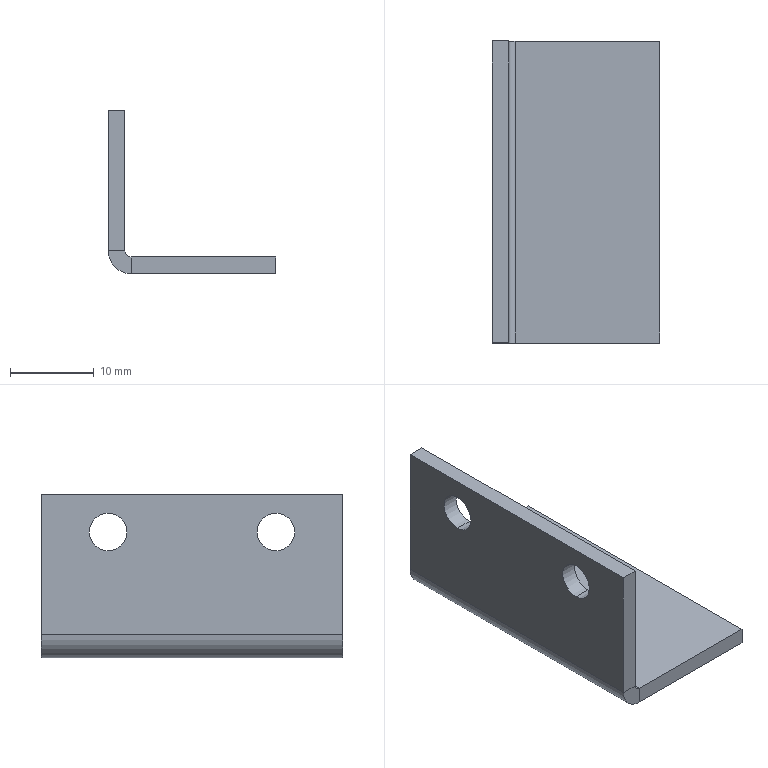Part | SolidWorks | features EdgeFlange 1, FlatPattern 1, HoleWzd 1, SMBaseFlange 1, SheetMetal 1 | 1 solid | 18 faces | box 20 x 36 x 19.5 mm | volume 2583 mm3 | plane 12 | cylinder 6 | commonest cylinder face diameters 4.5 x4 1.473 x1 5.473 x1
STEP:
#1=CARTESIAN_POINT('',(-10.,10.,15.25));
#2=VERTEX_POINT('',#1);
#3=CARTESIAN_POINT('',(-10.,10.,10.75));
#4=VERTEX_POINT('',#3);
#5=CARTESIAN_POINT('',(-10.,10.,13.));
#6=DIRECTION('',(1.,0.,0.));
#7=DIRECTION('',(0.,0.,-1.));
#8=AXIS2_PLACEMENT_3D('',#5,#6,#7);
#9=CIRCLE('',#8,2.25);
#10=EDGE_CURVE('',#2,#4,#9,.T.);
#11=ORIENTED_EDGE('',*,*,#10,.F.);
#12=CARTESIAN_POINT('',(-8.,10.,15.25));
#13=VERTEX_POINT('',#12);
#14=CARTESIAN_POINT('',(-8.,10.,15.25));
#15=DIRECTION('',(1.,0.,0.));
#16=VECTOR('',#15,1000.);
#17=LINE('',#14,#16);
#18=EDGE_CURVE('',#2,#13,#17,.T.);
#19=ORIENTED_EDGE('',*,*,#18,.T.);
#20=CARTESIAN_POINT('',(-8.,10.,10.75));
#21=VERTEX_POINT('',#20);
#22=CARTESIAN_POINT('',(-8.,10.,13.));
#23=DIRECTION('',(1.,0.,0.));
#24=DIRECTION('',(0.,0.,-1.));
#25=AXIS2_PLACEMENT_3D('',#22,#23,#24);
#26=CIRCLE('',#25,2.25);
#27=EDGE_CURVE('',#13,#21,#26,.T.);
#28=ORIENTED_EDGE('',*,*,#27,.T.);
#29=CARTESIAN_POINT('',(-8.,10.,10.75));
#30=DIRECTION('',(1.,0.,0.));
#31=VECTOR('',#30,1000.);
#32=LINE('',#29,#31);
#33=EDGE_CURVE('',#4,#21,#32,.T.);
#34=ORIENTED_EDGE('',*,*,#33,.F.);
#35=EDGE_LOOP('',(#11,#19,#28,#34));
#36=FACE_OUTER_BOUND('',#35,.T.);
#37=CARTESIAN_POINT('',(-8.,10.,13.));
#38=DIRECTION('',(1.,0.,0.));
#39=DIRECTION('',(0.,0.,-1.));
#40=AXIS2_PLACEMENT_3D('',#37,#38,#39);
#41=CYLINDRICAL_SURFACE('',#40,2.25);
#42=ADVANCED_FACE('',(#36),#41,.F.);
#43=CARTESIAN_POINT('',(-10.,-10.,15.25));
#44=VERTEX_POINT('',#43);
#45=CARTESIAN_POINT('',(-10.,-10.,10.75));
#46=VERTEX_POINT('',#45);
#47=CARTESIAN_POINT('',(-10.,-10.,13.));
#48=DIRECTION('',(1.,0.,0.));
#49=DIRECTION('',(0.,0.,-1.));
#50=AXIS2_PLACEMENT_3D('',#47,#48,#49);
#51=CIRCLE('',#50,2.25);
#52=EDGE_CURVE('',#44,#46,#51,.T.);
#53=ORIENTED_EDGE('',*,*,#52,.F.);
#54=CARTESIAN_POINT('',(-8.,-10.,15.25));
#55=VERTEX_POINT('',#54);
#56=CARTESIAN_POINT('',(-8.,-10.,15.25));
#57=DIRECTION('',(1.,0.,0.));
#58=VECTOR('',#57,1000.);
#59=LINE('',#56,#58);
#60=EDGE_CURVE('',#44,#55,#59,.T.);
#61=ORIENTED_EDGE('',*,*,#60,.T.);
#62=CARTESIAN_POINT('',(-8.,-10.,10.75));
#63=VERTEX_POINT('',#62);
#64=CARTESIAN_POINT('',(-8.,-10.,13.));
#65=DIRECTION('',(1.,0.,0.));
#66=DIRECTION('',(0.,0.,-1.));
#67=AXIS2_PLACEMENT_3D('',#64,#65,#66);
#68=CIRCLE('',#67,2.25);
#69=EDGE_CURVE('',#55,#63,#68,.T.);
#70=ORIENTED_EDGE('',*,*,#69,.T.);
#71=CARTESIAN_POINT('',(-8.,-10.,10.75));
#72=DIRECTION('',(1.,0.,0.));
#73=VECTOR('',#72,1000.);
#74=LINE('',#71,#73);
#75=EDGE_CURVE('',#46,#63,#74,.T.);
#76=ORIENTED_EDGE('',*,*,#75,.F.);
#77=EDGE_LOOP('',(#53,#61,#70,#76));
#78=FACE_OUTER_BOUND('',#77,.T.);
#79=CARTESIAN_POINT('',(-8.,-10.,13.));
#80=DIRECTION('',(1.,0.,0.));
#81=DIRECTION('',(0.,0.,-1.));
#82=AXIS2_PLACEMENT_3D('',#79,#80,#81);
#83=CYLINDRICAL_SURFACE('',#82,2.25);
#84=ADVANCED_FACE('',(#78),#83,.F.);
#85=CARTESIAN_POINT('',(-7.263,-18.,0.));
#86=VERTEX_POINT('',#85);
#87=CARTESIAN_POINT('',(10.,-18.,0.));
#88=VERTEX_POINT('',#87);
#89=CARTESIAN_POINT('',(-10.,-18.,0.));
#90=DIRECTION('',(1.,0.,0.));
#91=VECTOR('',#90,1000.);
#92=LINE('',#89,#91);
#93=EDGE_CURVE('',#86,#88,#92,.T.);
#94=ORIENTED_EDGE('',*,*,#93,.F.);
#95=CARTESIAN_POINT('',(-7.263,-18.,-2.));
#96=VERTEX_POINT('',#95);
#97=CARTESIAN_POINT('',(-7.263,-18.,0.));
#98=DIRECTION('',(0.,0.,-1.));
#99=VECTOR('',#98,1000.);
#100=LINE('',#97,#99);
#101=EDGE_CURVE('',#86,#96,#100,.T.);
#102=ORIENTED_EDGE('',*,*,#101,.T.);
#103=CARTESIAN_POINT('',(10.,-18.,-2.));
#104=VERTEX_POINT('',#103);
#105=CARTESIAN_POINT('',(-10.,-18.,-2.));
#106=DIRECTION('',(1.,0.,0.));
#107=VECTOR('',#106,1000.);
#108=LINE('',#105,#107);
#109=EDGE_CURVE('',#96,#104,#108,.T.);
#110=ORIENTED_EDGE('',*,*,#109,.T.);
#111=CARTESIAN_POINT('',(10.,-18.,-2.));
#112=DIRECTION('',(0.,0.,1.));
#113=VECTOR('',#112,1000.);
#114=LINE('',#111,#113);
#115=EDGE_CURVE('',#104,#88,#114,.T.);
#116=ORIENTED_EDGE('',*,*,#115,.T.);
#117=EDGE_LOOP('',(#94,#102,#110,#116));
#118=FACE_OUTER_BOUND('',#117,.T.);
#119=CARTESIAN_POINT('',(-10.,-18.,-2.));
#120=DIRECTION('',(0.,-1.,0.));
#121=DIRECTION('',(0.,0.,-1.));
#122=AXIS2_PLACEMENT_3D('',#119,#120,#121);
#123=PLANE('',#122);
#124=ADVANCED_FACE('',(#118),#123,.T.);
#125=CARTESIAN_POINT('',(-7.263,18.,-2.));
#126=VERTEX_POINT('',#125);
#127=CARTESIAN_POINT('',(-7.263,-18.,-2.));
#128=DIRECTION('',(0.,1.,0.));
#129=VECTOR('',#128,1000.);
#130=LINE('',#127,#129);
#131=EDGE_CURVE('',#96,#126,#130,.T.);
#132=ORIENTED_EDGE('',*,*,#131,.T.);
#133=CARTESIAN_POINT('',(10.,18.,-2.));
#134=VERTEX_POINT('',#133);
#135=CARTESIAN_POINT('',(-10.,18.,-2.));
#136=DIRECTION('',(-1.,0.,0.));
#137=VECTOR('',#136,1000.);
#138=LINE('',#135,#137);
#139=EDGE_CURVE('',#134,#126,#138,.T.);
#140=ORIENTED_EDGE('',*,*,#139,.F.);
#141=CARTESIAN_POINT('',(10.,18.,-2.));
#142=DIRECTION('',(0.,1.,0.));
#143=VECTOR('',#142,1000.);
#144=LINE('',#141,#143);
#145=EDGE_CURVE('',#104,#134,#144,.T.);
#146=ORIENTED_EDGE('',*,*,#145,.F.);
#147=ORIENTED_EDGE('',*,*,#109,.F.);
#148=EDGE_LOOP('',(#132,#140,#146,#147));
#149=FACE_OUTER_BOUND('',#148,.T.);
#150=CARTESIAN_POINT('',(0.,0.,-2.));
#151=DIRECTION('',(0.,0.,1.));
#152=DIRECTION('',(1.,0.,0.));
#153=AXIS2_PLACEMENT_3D('',#150,#151,#152);
#154=PLANE('',#153);
#155=ADVANCED_FACE('',(#149),#154,.F.);
#156=CARTESIAN_POINT('',(10.,18.,0.));
#157=VERTEX_POINT('',#156);
#158=CARTESIAN_POINT('',(-7.263,18.,0.));
#159=VERTEX_POINT('',#158);
#160=CARTESIAN_POINT('',(-10.,18.,0.));
#161=DIRECTION('',(-1.,0.,0.));
#162=VECTOR('',#161,1000.);
#163=LINE('',#160,#162);
#164=EDGE_CURVE('',#157,#159,#163,.T.);
#165=ORIENTED_EDGE('',*,*,#164,.T.);
#166=CARTESIAN_POINT('',(-7.263,-18.,0.));
#167=DIRECTION('',(0.,1.,0.));
#168=VECTOR('',#167,1000.);
#169=LINE('',#166,#168);
#170=EDGE_CURVE('',#86,#159,#169,.T.);
#171=ORIENTED_EDGE('',*,*,#170,.F.);
#172=ORIENTED_EDGE('',*,*,#93,.T.);
#173=CARTESIAN_POINT('',(10.,18.,0.));
#174=DIRECTION('',(0.,1.,0.));
#175=VECTOR('',#174,1000.);
#176=LINE('',#173,#175);
#177=EDGE_CURVE('',#88,#157,#176,.T.);
#178=ORIENTED_EDGE('',*,*,#177,.T.);
#179=EDGE_LOOP('',(#165,#171,#172,#178));
#180=FACE_OUTER_BOUND('',#179,.T.);
#181=CARTESIAN_POINT('',(0.,0.,0.));
#182=DIRECTION('',(0.,0.,1.));
#183=DIRECTION('',(1.,0.,0.));
#184=AXIS2_PLACEMENT_3D('',#181,#182,#183);
#185=PLANE('',#184);
#186=ADVANCED_FACE('',(#180),#185,.T.);
#187=ORIENTED_EDGE('',*,*,#177,.F.);
#188=ORIENTED_EDGE('',*,*,#115,.F.);
#189=ORIENTED_EDGE('',*,*,#145,.T.);
#190=CARTESIAN_POINT('',(10.,18.,-2.));
#191=DIRECTION('',(0.,0.,1.));
#192=VECTOR('',#191,1000.);
#193=LINE('',#190,#192);
#194=EDGE_CURVE('',#134,#157,#193,.T.);
#195=ORIENTED_EDGE('',*,*,#194,.T.);
#196=EDGE_LOOP('',(#187,#188,#189,#195));
#197=FACE_OUTER_BOUND('',#196,.T.);
#198=CARTESIAN_POINT('',(10.,18.,-2.));
#199=DIRECTION('',(1.,0.,0.));
#200=DIRECTION('',(0.,1.,0.));
#201=AXIS2_PLACEMENT_3D('',#198,#199,#200);
#202=PLANE('',#201);
#203=ADVANCED_FACE('',(#197),#202,.T.);
#204=CARTESIAN_POINT('',(-7.263,18.,0.));
#205=DIRECTION('',(0.,0.,-1.));
#206=VECTOR('',#205,1000.);
#207=LINE('',#204,#206);
#208=EDGE_CURVE('',#159,#126,#207,.T.);
#209=ORIENTED_EDGE('',*,*,#208,.F.);
#210=ORIENTED_EDGE('',*,*,#164,.F.);
#211=ORIENTED_EDGE('',*,*,#194,.F.);
#212=ORIENTED_EDGE('',*,*,#139,.T.);
#213=EDGE_LOOP('',(#209,#210,#211,#212));
#214=FACE_OUTER_BOUND('',#213,.T.);
#215=CARTESIAN_POINT('',(-10.,18.,-2.));
#216=DIRECTION('',(0.,1.,0.));
#217=DIRECTION('',(0.,0.,1.));
#218=AXIS2_PLACEMENT_3D('',#215,#216,#217);
#219=PLANE('',#218);
#220=ADVANCED_FACE('',(#214),#219,.T.);
#221=CARTESIAN_POINT('',(-8.,18.,0.7366));
#222=VERTEX_POINT('',#221);
#223=CARTESIAN_POINT('',(-10.,18.,0.7366));
#224=VERTEX_POINT('',#223);
#225=CARTESIAN_POINT('',(-10.,18.,0.7366));
#226=DIRECTION('',(-1.,0.,0.));
#227=VECTOR('',#226,1000.);
#228=LINE('',#225,#227);
#229=EDGE_CURVE('',#222,#224,#228,.T.);
#230=ORIENTED_EDGE('',*,*,#229,.F.);
#231=CARTESIAN_POINT('',(-7.263,18.,0.7366));
#232=DIRECTION('',(0.,1.,0.));
#233=DIRECTION('',(0.,0.,-1.));
#234=AXIS2_PLACEMENT_3D('',#231,#232,#233);
#235=CIRCLE('',#234,0.7366);
#236=EDGE_CURVE('',#159,#222,#235,.T.);
#237=ORIENTED_EDGE('',*,*,#236,.F.);
#238=ORIENTED_EDGE('',*,*,#208,.T.);
#239=CARTESIAN_POINT('',(-7.263,18.,0.7366));
#240=DIRECTION('',(0.,1.,0.));
#241=DIRECTION('',(0.,0.,-1.));
#242=AXIS2_PLACEMENT_3D('',#239,#240,#241);
#243=CIRCLE('',#242,2.737);
#244=EDGE_CURVE('',#126,#224,#243,.T.);
#245=ORIENTED_EDGE('',*,*,#244,.T.);
#246=EDGE_LOOP('',(#230,#237,#238,#245));
#247=FACE_OUTER_BOUND('',#246,.T.);
#248=CARTESIAN_POINT('',(-7.263,18.,0.7366));
#249=DIRECTION('',(0.,1.,0.));
#250=DIRECTION('',(0.,0.,1.));
#251=AXIS2_PLACEMENT_3D('',#248,#249,#250);
#252=PLANE('',#251);
#253=ADVANCED_FACE('',(#247),#252,.T.);
#254=CARTESIAN_POINT('',(-8.,-18.,0.7366));
#255=VERTEX_POINT('',#254);
#256=CARTESIAN_POINT('',(-7.263,-18.,0.7366));
#257=DIRECTION('',(0.,-1.,0.));
#258=DIRECTION('',(0.,0.,-1.));
#259=AXIS2_PLACEMENT_3D('',#256,#257,#258);
#260=CIRCLE('',#259,0.7366);
#261=EDGE_CURVE('',#255,#86,#260,.T.);
#262=ORIENTED_EDGE('',*,*,#261,.F.);
#263=CARTESIAN_POINT('',(-10.,-18.,0.7366));
#264=VERTEX_POINT('',#263);
#265=CARTESIAN_POINT('',(-8.,-18.,0.7366));
#266=DIRECTION('',(-1.,0.,0.));
#267=VECTOR('',#266,1000.);
#268=LINE('',#265,#267);
#269=EDGE_CURVE('',#255,#264,#268,.T.);
#270=ORIENTED_EDGE('',*,*,#269,.T.);
#271=CARTESIAN_POINT('',(-7.263,-18.,0.7366));
#272=DIRECTION('',(0.,-1.,0.));
#273=DIRECTION('',(0.,0.,-1.));
#274=AXIS2_PLACEMENT_3D('',#271,#272,#273);
#275=CIRCLE('',#274,2.737);
#276=EDGE_CURVE('',#264,#96,#275,.T.);
#277=ORIENTED_EDGE('',*,*,#276,.T.);
#278=ORIENTED_EDGE('',*,*,#101,.F.);
#279=EDGE_LOOP('',(#262,#270,#277,#278));
#280=FACE_OUTER_BOUND('',#279,.T.);
#281=CARTESIAN_POINT('',(-7.263,-18.,0.7366));
#282=DIRECTION('',(0.,1.,0.));
#283=DIRECTION('',(0.,0.,1.));
#284=AXIS2_PLACEMENT_3D('',#281,#282,#283);
#285=PLANE('',#284);
#286=ADVANCED_FACE('',(#280),#285,.F.);
#287=ORIENTED_EDGE('',*,*,#131,.F.);
#288=ORIENTED_EDGE('',*,*,#276,.F.);
#289=CARTESIAN_POINT('',(-10.,18.,0.7366));
#290=DIRECTION('',(0.,1.,0.));
#291=VECTOR('',#290,1000.);
#292=LINE('',#289,#291);
#293=EDGE_CURVE('',#264,#224,#292,.T.);
#294=ORIENTED_EDGE('',*,*,#293,.T.);
#295=ORIENTED_EDGE('',*,*,#244,.F.);
#296=EDGE_LOOP('',(#287,#288,#294,#295));
#297=FACE_OUTER_BOUND('',#296,.T.);
#298=CARTESIAN_POINT('',(-7.263,-18.,0.7366));
#299=DIRECTION('',(0.,-1.,0.));
#300=DIRECTION('',(-1.,0.,0.));
#301=AXIS2_PLACEMENT_3D('',#298,#299,#300);
#302=CYLINDRICAL_SURFACE('',#301,2.737);
#303=ADVANCED_FACE('',(#297),#302,.T.);
#304=ORIENTED_EDGE('',*,*,#170,.T.);
#305=ORIENTED_EDGE('',*,*,#236,.T.);
#306=CARTESIAN_POINT('',(-8.,18.,0.7366));
#307=DIRECTION('',(0.,-1.,0.));
#308=VECTOR('',#307,1000.);
#309=LINE('',#306,#308);
#310=EDGE_CURVE('',#222,#255,#309,.T.);
#311=ORIENTED_EDGE('',*,*,#310,.T.);
#312=ORIENTED_EDGE('',*,*,#261,.T.);
#313=EDGE_LOOP('',(#304,#305,#311,#312));
#314=FACE_OUTER_BOUND('',#313,.T.);
#315=CARTESIAN_POINT('',(-7.263,-18.,0.7366));
#316=DIRECTION('',(0.,-1.,0.));
#317=DIRECTION('',(-1.,0.,0.));
#318=AXIS2_PLACEMENT_3D('',#315,#316,#317);
#319=CYLINDRICAL_SURFACE('',#318,0.7366);
#320=ADVANCED_FACE('',(#314),#319,.F.);
#321=ORIENTED_EDGE('',*,*,#229,.T.);
#322=CARTESIAN_POINT('',(-10.,18.,17.5));
#323=VERTEX_POINT('',#322);
#324=CARTESIAN_POINT('',(-10.,18.,0.));
#325=DIRECTION('',(0.,0.,-1.));
#326=VECTOR('',#325,1000.);
#327=LINE('',#324,#326);
#328=EDGE_CURVE('',#323,#224,#327,.T.);
#329=ORIENTED_EDGE('',*,*,#328,.F.);
#330=CARTESIAN_POINT('',(-8.,18.,17.5));
#331=VERTEX_POINT('',#330);
#332=CARTESIAN_POINT('',(-10.,18.,17.5));
#333=DIRECTION('',(1.,0.,0.));
#334=VECTOR('',#333,1000.);
#335=LINE('',#332,#334);
#336=EDGE_CURVE('',#323,#331,#335,.T.);
#337=ORIENTED_EDGE('',*,*,#336,.T.);
#338=CARTESIAN_POINT('',(-8.,18.,0.));
#339=DIRECTION('',(0.,0.,-1.));
#340=VECTOR('',#339,1000.);
#341=LINE('',#338,#340);
#342=EDGE_CURVE('',#331,#222,#341,.T.);
#343=ORIENTED_EDGE('',*,*,#342,.T.);
#344=EDGE_LOOP('',(#321,#329,#337,#343));
#345=FACE_OUTER_BOUND('',#344,.T.);
#346=CARTESIAN_POINT('',(-10.,18.,0.));
#347=DIRECTION('',(0.,-1.,0.));
#348=DIRECTION('',(1.,0.,0.));
#349=AXIS2_PLACEMENT_3D('',#346,#347,#348);
#350=PLANE('',#349);
#351=ADVANCED_FACE('',(#345),#350,.F.);
#352=ORIENTED_EDGE('',*,*,#269,.F.);
#353=CARTESIAN_POINT('',(-8.,-18.,17.5));
#354=VERTEX_POINT('',#353);
#355=CARTESIAN_POINT('',(-8.,-18.,17.5));
#356=DIRECTION('',(0.,0.,1.));
#357=VECTOR('',#356,1000.);
#358=LINE('',#355,#357);
#359=EDGE_CURVE('',#255,#354,#358,.T.);
#360=ORIENTED_EDGE('',*,*,#359,.T.);
#361=CARTESIAN_POINT('',(-10.,-18.,17.5));
#362=VERTEX_POINT('',#361);
#363=CARTESIAN_POINT('',(-10.,-18.,17.5));
#364=DIRECTION('',(1.,0.,0.));
#365=VECTOR('',#364,1000.);
#366=LINE('',#363,#365);
#367=EDGE_CURVE('',#362,#354,#366,.T.);
#368=ORIENTED_EDGE('',*,*,#367,.F.);
#369=CARTESIAN_POINT('',(-10.,-18.,0.));
#370=DIRECTION('',(0.,0.,1.));
#371=VECTOR('',#370,1000.);
#372=LINE('',#369,#371);
#373=EDGE_CURVE('',#264,#362,#372,.T.);
#374=ORIENTED_EDGE('',*,*,#373,.F.);
#375=EDGE_LOOP('',(#352,#360,#368,#374));
#376=FACE_OUTER_BOUND('',#375,.T.);
#377=CARTESIAN_POINT('',(-10.,-18.,17.5));
#378=DIRECTION('',(0.,1.,0.));
#379=DIRECTION('',(-1.,0.,0.));
#380=AXIS2_PLACEMENT_3D('',#377,#378,#379);
#381=PLANE('',#380);
#382=ADVANCED_FACE('',(#376),#381,.F.);
#383=CARTESIAN_POINT('',(-10.,10.,13.));
#384=DIRECTION('',(1.,0.,0.));
#385=DIRECTION('',(0.,0.,-1.));
#386=AXIS2_PLACEMENT_3D('',#383,#384,#385);
#387=CIRCLE('',#386,2.25);
#388=EDGE_CURVE('',#4,#2,#387,.T.);
#389=ORIENTED_EDGE('',*,*,#388,.T.);
#390=ORIENTED_EDGE('',*,*,#10,.T.);
#391=EDGE_LOOP('',(#389,#390));
#392=FACE_BOUND('',#391,.T.);
#393=CARTESIAN_POINT('',(-10.,-10.,13.));
#394=DIRECTION('',(1.,0.,0.));
#395=DIRECTION('',(0.,0.,-1.));
#396=AXIS2_PLACEMENT_3D('',#393,#394,#395);
#397=CIRCLE('',#396,2.25);
#398=EDGE_CURVE('',#46,#44,#397,.T.);
#399=ORIENTED_EDGE('',*,*,#398,.T.);
#400=ORIENTED_EDGE('',*,*,#52,.T.);
#401=EDGE_LOOP('',(#399,#400));
#402=FACE_BOUND('',#401,.T.);
#403=ORIENTED_EDGE('',*,*,#293,.F.);
#404=ORIENTED_EDGE('',*,*,#373,.T.);
#405=CARTESIAN_POINT('',(-10.,0.,17.5));
#406=DIRECTION('',(0.,1.,0.));
#407=VECTOR('',#406,1000.);
#408=LINE('',#405,#407);
#409=EDGE_CURVE('',#362,#323,#408,.T.);
#410=ORIENTED_EDGE('',*,*,#409,.T.);
#411=ORIENTED_EDGE('',*,*,#328,.T.);
#412=EDGE_LOOP('',(#403,#404,#410,#411));
#413=FACE_OUTER_BOUND('',#412,.T.);
#414=CARTESIAN_POINT('',(-10.,0.,0.));
#415=DIRECTION('',(1.,0.,0.));
#416=DIRECTION('',(0.,0.,-1.));
#417=AXIS2_PLACEMENT_3D('',#414,#415,#416);
#418=PLANE('',#417);
#419=ADVANCED_FACE('',(#392,#402,#413),#418,.F.);
#420=CARTESIAN_POINT('',(-8.,10.,13.));
#421=DIRECTION('',(1.,0.,0.));
#422=DIRECTION('',(0.,0.,-1.));
#423=AXIS2_PLACEMENT_3D('',#420,#421,#422);
#424=CIRCLE('',#423,2.25);
#425=EDGE_CURVE('',#21,#13,#424,.T.);
#426=ORIENTED_EDGE('',*,*,#425,.F.);
#427=ORIENTED_EDGE('',*,*,#27,.F.);
#428=EDGE_LOOP('',(#426,#427));
#429=FACE_BOUND('',#428,.T.);
#430=CARTESIAN_POINT('',(-8.,-10.,13.));
#431=DIRECTION('',(1.,0.,0.));
#432=DIRECTION('',(0.,0.,-1.));
#433=AXIS2_PLACEMENT_3D('',#430,#431,#432);
#434=CIRCLE('',#433,2.25);
#435=EDGE_CURVE('',#63,#55,#434,.T.);
#436=ORIENTED_EDGE('',*,*,#435,.F.);
#437=ORIENTED_EDGE('',*,*,#69,.F.);
#438=EDGE_LOOP('',(#436,#437));
#439=FACE_BOUND('',#438,.T.);
#440=ORIENTED_EDGE('',*,*,#359,.F.);
#441=ORIENTED_EDGE('',*,*,#310,.F.);
#442=ORIENTED_EDGE('',*,*,#342,.F.);
#443=CARTESIAN_POINT('',(-8.,18.,17.5));
#444=DIRECTION('',(0.,1.,0.));
#445=VECTOR('',#444,1000.);
#446=LINE('',#443,#445);
#447=EDGE_CURVE('',#354,#331,#446,.T.);
#448=ORIENTED_EDGE('',*,*,#447,.F.);
#449=EDGE_LOOP('',(#440,#441,#442,#448));
#450=FACE_OUTER_BOUND('',#449,.T.);
#451=CARTESIAN_POINT('',(-8.,0.,0.));
#452=DIRECTION('',(1.,0.,0.));
#453=DIRECTION('',(0.,0.,-1.));
#454=AXIS2_PLACEMENT_3D('',#451,#452,#453);
#455=PLANE('',#454);
#456=ADVANCED_FACE('',(#429,#439,#450),#455,.T.);
#457=ORIENTED_EDGE('',*,*,#447,.T.);
#458=ORIENTED_EDGE('',*,*,#336,.F.);
#459=ORIENTED_EDGE('',*,*,#409,.F.);
#460=ORIENTED_EDGE('',*,*,#367,.T.);
#461=EDGE_LOOP('',(#457,#458,#459,#460));
#462=FACE_OUTER_BOUND('',#461,.T.);
#463=CARTESIAN_POINT('',(-10.,18.,17.5));
#464=DIRECTION('',(0.,0.,-1.));
#465=DIRECTION('',(-1.,0.,0.));
#466=AXIS2_PLACEMENT_3D('',#463,#464,#465);
#467=PLANE('',#466);
#468=ADVANCED_FACE('',(#462),#467,.F.);
#469=ORIENTED_EDGE('',*,*,#60,.F.);
#470=ORIENTED_EDGE('',*,*,#398,.F.);
#471=ORIENTED_EDGE('',*,*,#75,.T.);
#472=ORIENTED_EDGE('',*,*,#435,.T.);
#473=EDGE_LOOP('',(#469,#470,#471,#472));
#474=FACE_OUTER_BOUND('',#473,.T.);
#475=CARTESIAN_POINT('',(-8.,-10.,13.));
#476=DIRECTION('',(1.,0.,0.));
#477=DIRECTION('',(0.,0.,-1.));
#478=AXIS2_PLACEMENT_3D('',#475,#476,#477);
#479=CYLINDRICAL_SURFACE('',#478,2.25);
#480=ADVANCED_FACE('',(#474),#479,.F.);
#481=ORIENTED_EDGE('',*,*,#18,.F.);
#482=ORIENTED_EDGE('',*,*,#388,.F.);
#483=ORIENTED_EDGE('',*,*,#33,.T.);
#484=ORIENTED_EDGE('',*,*,#425,.T.);
#485=EDGE_LOOP('',(#481,#482,#483,#484));
#486=FACE_OUTER_BOUND('',#485,.T.);
#487=CARTESIAN_POINT('',(-8.,10.,13.));
#488=DIRECTION('',(1.,0.,0.));
#489=DIRECTION('',(0.,0.,-1.));
#490=AXIS2_PLACEMENT_3D('',#487,#488,#489);
#491=CYLINDRICAL_SURFACE('',#490,2.25);
#492=ADVANCED_FACE('',(#486),#491,.F.);
#493=CLOSED_SHELL('',(#42,#84,#124,#155,#186,#203,#220,#253,#286,#303,#320,#351,#382,#419,#456,#468,#480,#492));
#494=MANIFOLD_SOLID_BREP('',#493);
#495=CARTESIAN_POINT('',(0.,0.,0.));
#496=DIRECTION('',(0.,0.,1.));
#497=DIRECTION('',(1.,0.,0.));
#498=AXIS2_PLACEMENT_3D('',#495,#496,#497);
#499=(LENGTH_UNIT()NAMED_UNIT(*)SI_UNIT(.MILLI.,.METRE.));
#500=UNCERTAINTY_MEASURE_WITH_UNIT(LENGTH_MEASURE(0.00001),#499,'','');
#501=(NAMED_UNIT(*)PLANE_ANGLE_UNIT()SI_UNIT($,.RADIAN.));
#502=(NAMED_UNIT(*)SI_UNIT($,.STERADIAN.)SOLID_ANGLE_UNIT());
#503=(GEOMETRIC_REPRESENTATION_CONTEXT(3)GLOBAL_UNCERTAINTY_ASSIGNED_CONTEXT((#500))GLOBAL_UNIT_ASSIGNED_CONTEXT((#499,#501,#502))REPRESENTATION_CONTEXT('',''));
#504=ADVANCED_BREP_SHAPE_REPRESENTATION('',(#494,#498),#503);